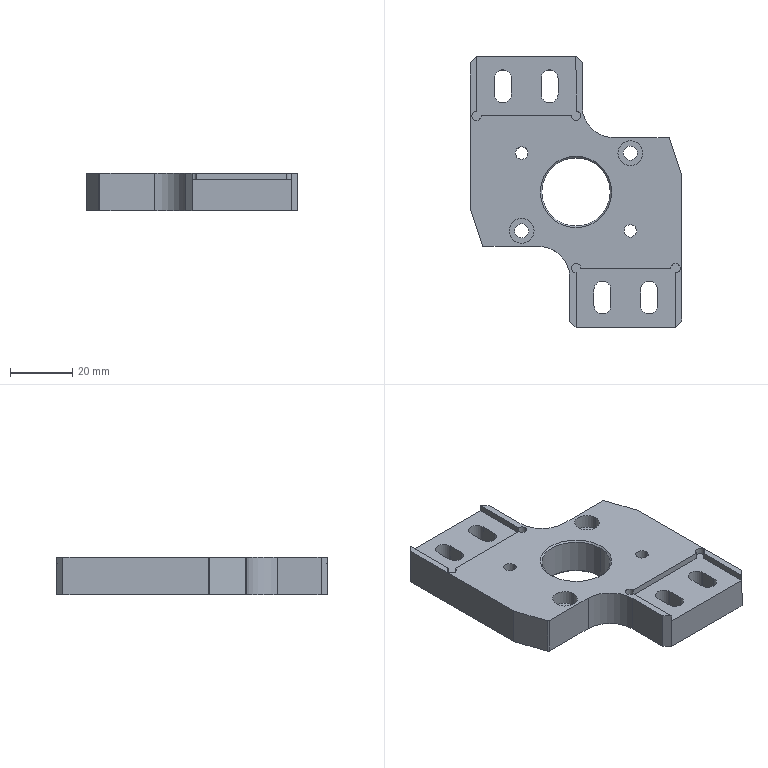Part | SolidWorks | features Chamfer 3, Fillet 2, ICE 2, Cut 1, Extrusion 1, HoleWzd 1 | 1 solid | 72 faces | box 68 x 87 x 12 mm | volume 40763 mm3 | cylinder 34 | plane 34 | cone 4 | commonest cylinder face diameters 5.5 x8 3 x6 1 x4 4 x4 4.5 x4 8 x4